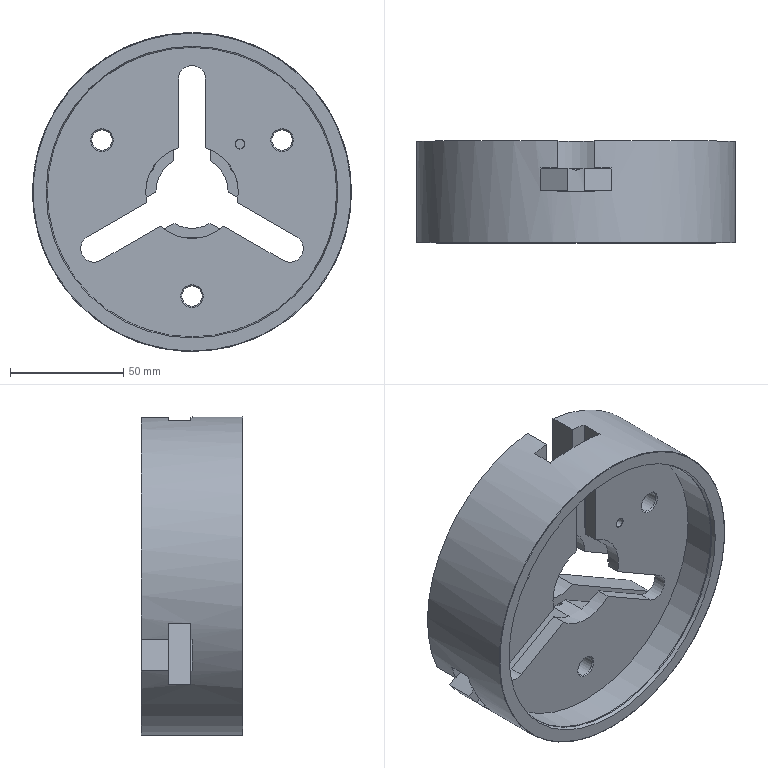NC program | NX | posted with a generic post | part box 141 x 45 x 141 mm
Whole program:
N10 G17 G21 G94 G90
(PLANAR_MILL_COPY_2 , TOOL : D14)
N12 T05 M6
N14 G54
N16 G17 G0 G90 X0. Y89. S3600 M3
N18 G43 Z100. H5
N20 Z-21.5
N22 G41 G94 G1 Z-22.5 F3600. D4
N24 Y75.
N26 X1.
N28 Y7.
N30 X-1.
N32 Y75.
N34 X0.
N36 G40
N38 Y89.
N40 Z-21.5
N42 G0 Z100.
(PLANAR_MILL_COPY_2_COPY , TOOL : D14)
N44 X-77.076 Y-44.5
N46 Z-21.5
N48 G41 G1 Z-22.5
N50 X-64.952 Y-37.5
N52 X-65.452 Y-36.634
N54 X-6.562 Y-2.634
N56 X-5.562 Y-4.366
N58 X-64.452 Y-38.366
N60 X-64.952 Y-37.5
N62 G40
N64 X-77.076 Y-44.5
N66 Z-21.5
N68 G0 Z100.
(PLANAR_MILL_COPY_2_COPY_1 , TOOL : D14)
N70 X77.076
N72 Z-21.5
N74 G41 G1 Z-22.5
N76 X64.952 Y-37.5
N78 X64.452 Y-38.366
N80 X5.562 Y-4.366
N82 X6.562 Y-2.634
N84 X65.452 Y-36.634
N86 X64.952 Y-37.5
N88 G40
N90 X77.076 Y-44.5
N92 Z-21.5
N94 G0 Z100.
N96 M5
N98 M2